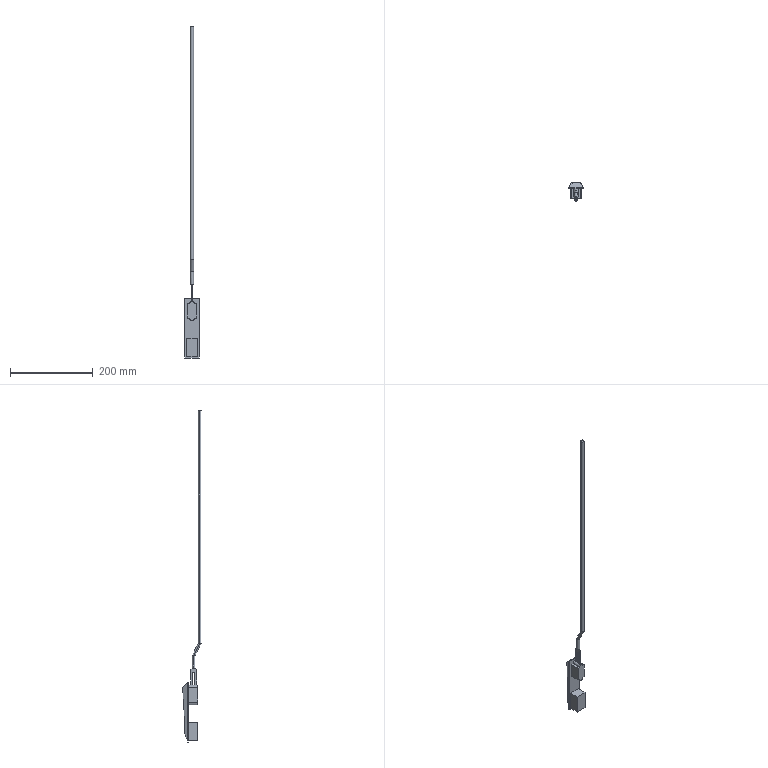Part | NX | features solid 2 | 1 solid | 93 faces | box 36 x 45 x 804 mm | volume 122528 mm3 | plane 55 | cylinder 34 | cone 2 | spline 2 | commonest cylinder face diameters 6.1 x20 2 x4 8 x4 1 x3 10 x2 3 x1